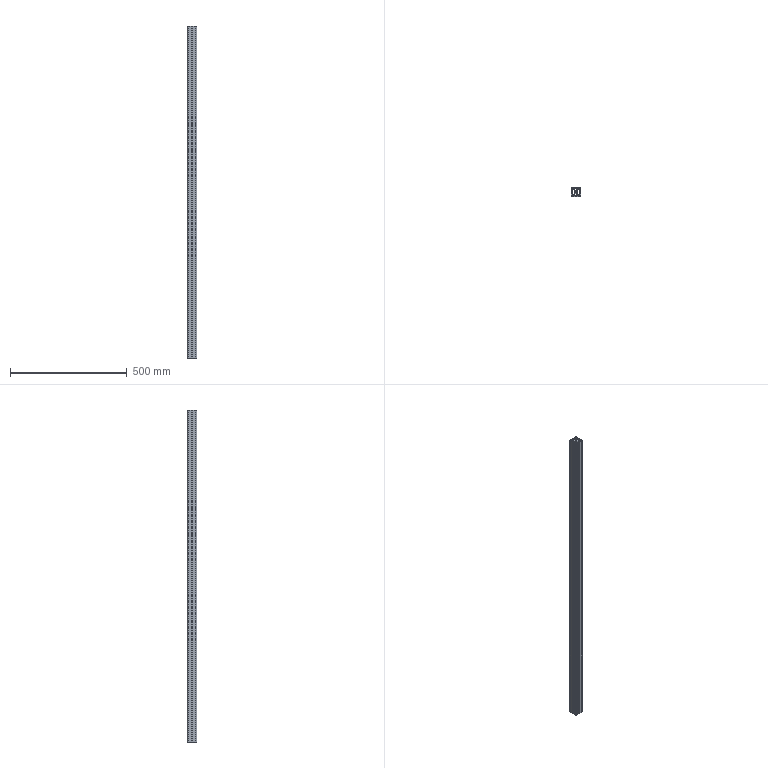Part | STEP file | 40x40-1420 | 1 solid | 88 faces | box 40 x 40 x 1420 mm | volume 999605 mm3 | plane 78 | cylinder 10 | commonest cylinder face diameters 4 x4 10 x4 6.8 x2